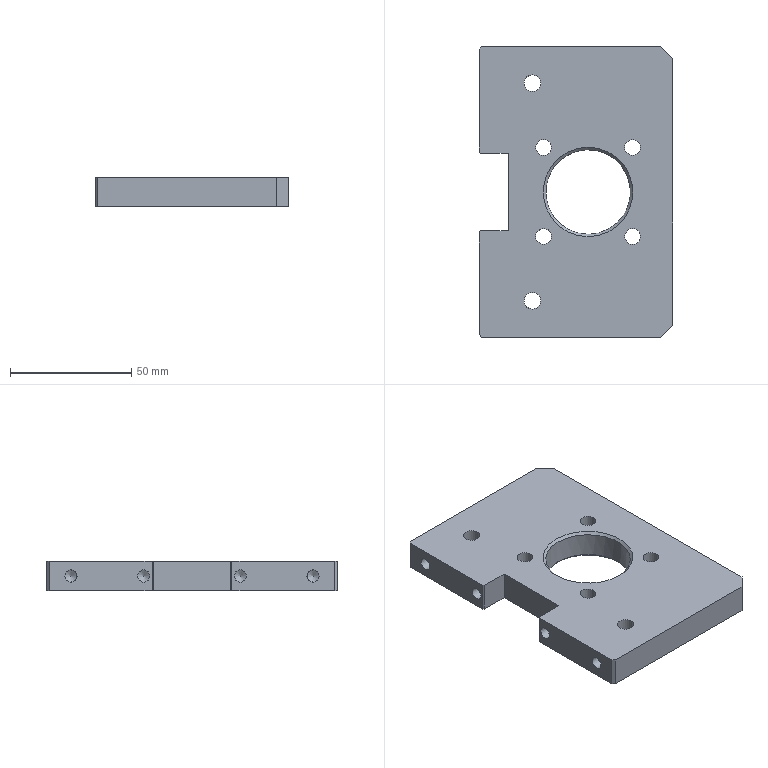NC program | NX | posted with a generic post | part box 80 x 120 x 12 mm
Whole program:
N10 G17 G21 G94 G90
(DRILLING , TOOL : D8A45)
N12 T06 M6
N14 G54
N16 G17 G0 G90 X-50. Y0. B0. C0. S3500 M3
N18 G43 Z30. H6
N20 G94 G81 G98 Z-2.6 F250. R3.
N22 X-20.
N24 X20.
N26 X50.
N28 G80
N30 G0 X50. Y0. Z30.
N32 M5
(DRILLING_1 , TOOL : 5.0ZT)
N34 T14 M6
N36 G54
N38 G17 G0 G90 X-50. Y0. B0. C0. S2000 M3
N40 G43 Z30. H14
N42 G94 G83 G98 Z-21.443 F200. Q3. R3.
N44 X-20.
N46 X20.
N48 X50.
N50 G80
N52 G0 X50. Y0. Z30.
N54 M5
(FLOOR_WALL_1 , TOOL : D10)
N56 T04 M6
N58 G54
N60 G17 G0 G90 X-1. Y12.5 B0. C0. S7000 M3
N62 G43 Z30. H4
N64 Z0.508
N66 G94 G1 Z-0.992 F1000.
N68 Y7.
N70 G3 X0. Y6. R1.
N72 G1 X10.9 F3000.
N74 Y-6.
N76 X-10.9
N78 Y6.
N80 X0.
N82 Y1.5
N84 X6.4
N86 Y-1.5
N88 X-6.4
N90 Y1.5
N92 X0.
N94 G3 X1. Y2.5 R1.
N96 G1 Z0.508
N98 G0 X-1. Y12.5 Z-0.483
N100 G1 Z-1.983 F1000.
N102 Y7.
N104 G3 X0. Y6. R1.
N106 G1 X10.9 F3000.
N108 Y-6.
N110 X-10.9
N112 Y6.
N114 X0.
N116 Y1.5
N118 X6.4
N120 Y-1.5
N122 X-6.4
N124 Y1.5
N126 X0.
N128 G3 X1. Y2.5 R1.
N130 G1 Z-0.483
N132 G0 X-1. Y12.5 Z-1.475
N134 G1 Z-2.975 F1000.
N136 Y7.
N138 G3 X0. Y6. R1.
N140 G1 X10.9 F3000.
N142 Y-6.
N144 X-10.9
N146 Y6.
N148 X0.
N150 Y1.5
N152 X6.4
N154 Y-1.5
N156 X-6.4
N158 Y1.5
N160 X0.
N162 G3 X1. Y2.5 R1.
N164 G1 Z-1.475
N166 G0 X-1. Y12.5 Z-2.467
N168 G1 Z-3.967 F1000.
N170 Y7.
N172 G3 X0. Y6. R1.
N174 G1 X10.9 F3000.
N176 Y-6.
N178 X-10.9
N180 Y6.
N182 X0.
N184 Y1.5
N186 X6.4
N188 Y-1.5
N190 X-6.4
N192 Y1.5
N194 X0.
N196 G3 X1. Y2.5 R1.
N198 G1 Z-2.467
N200 G0 X-1. Y12.5 Z-3.458
N202 G1 Z-4.958 F1000.
N204 Y7.
N206 G3 X0. Y6. R1.
N208 G1 X10.9 F3000.
N210 Y-6.
N212 X-10.9
N214 Y6.
N216 X0.
N218 Y1.5
N220 X6.4
N222 Y-1.5
N224 X-6.4
N226 Y1.5
N228 X0.
N230 G3 X1. Y2.5 R1.
N232 G1 Z-3.458
N234 G0 X-1. Y12.5 Z-4.45
N236 G1 Z-5.95 F1000.
N238 Y7.
N240 G3 X0. Y6. R1.
N242 G1 X10.9 F3000.
N244 Y-6.
N246 X-10.9
N248 Y6.
N250 X0.
N252 Y1.5
N254 X6.4
N256 Y-1.5
N258 X-6.4
N260 Y1.5
N262 X0.
N264 G3 X1. Y2.5 R1.
N266 G1 Z-4.45
N268 G0 X-1. Y12.5 Z-5.442
N270 G1 Z-6.942 F1000.
N272 Y7.
N274 G3 X0. Y6. R1.
N276 G1 X10.9 F3000.
N278 Y-6.
N280 X-10.9
N282 Y6.
N284 X0.
N286 Y1.5
N288 X6.4
N290 Y-1.5
N292 X-6.4
N294 Y1.5
N296 X0.
N298 G3 X1. Y2.5 R1.
N300 G1 Z-5.442
N302 G0 X-1. Y12.5 Z-6.433
N304 G1 Z-7.933 F1000.
N306 Y7.
N308 G3 X0. Y6. R1.
N310 G1 X10.9 F3000.
N312 Y-6.
N314 X-10.9
N316 Y6.
N318 X0.
N320 Y1.5
N322 X6.4
N324 Y-1.5
N326 X-6.4
N328 Y1.5
N330 X0.
N332 G3 X1. Y2.5 R1.
N334 G1 Z-6.433
N336 G0 X-1. Y12.5 Z-7.425
N338 G1 Z-8.925 F1000.
N340 Y7.
N342 G3 X0. Y6. R1.
N344 G1 X10.9 F3000.
N346 Y-6.
N348 X-10.9
N350 Y6.
N352 X0.
N354 Y1.5
N356 X6.4
N358 Y-1.5
N360 X-6.4
N362 Y1.5
N364 X0.
N366 G3 X1. Y2.5 R1.
N368 G1 Z-7.425
N370 G0 X-1. Y12.5 Z-8.417
N372 G1 Z-9.917 F1000.
N374 Y7.
N376 G3 X0. Y6. R1.
N378 G1 X10.9 F3000.
N380 Y-6.
N382 X-10.9
N384 Y6.
N386 X0.
N388 Y1.5
N390 X6.4
N392 Y-1.5
N394 X-6.4
N396 Y1.5
N398 X0.
N400 G3 X1. Y2.5 R1.
N402 G1 Z-8.417
N404 G0 X-1. Y12.5 Z-9.408
N406 G1 Z-10.908 F1000.
N408 Y7.
N410 G3 X0. Y6. R1.
N412 G1 X10.9 F3000.
N414 Y-6.
N416 X-10.9
N418 Y6.
N420 X0.
N422 Y1.5
N424 X6.4
N426 Y-1.5
N428 X-6.4
N430 Y1.5
N432 X0.
N434 G3 X1. Y2.5 R1.
N436 G1 Z-9.408
N438 G0 X-1. Y12.5 Z-10.4
N440 G1 Z-11.9 F1000.
N442 Y7.
N444 G3 X0. Y6. R1.
N446 G1 X10.9 F3000.
N448 Y-6.
N450 X-10.9
N452 Y6.
N454 X0.
N456 Y1.5
N458 X6.4
N460 Y-1.5
N462 X-6.4
N464 Y1.5
N466 X0.
N468 G3 X1. Y2.5 R1.
N470 G1 Z-10.4
N472 G0 Z30.
(FLOOR_WALL_1_COPY , TOOL : D10)
N474 X-9.497 Y-12.5
N476 Z-10.5
N478 G1 Z-12. F1000.
N480 Y-10.
N482 G3 X-10.497 Y-11. R1.
N484 G1 Y11. F1200.
N486 X-6.298
N488 Y-11.
N490 X-2.098
N492 Y11.
N494 X2.101
N496 Y-11.
N498 X6.301
N500 Y11.
N502 X10.5
N504 Y-11.
N506 G2 X9.5 Y-12. R1.
N508 G1 Y-12.5
N510 Z-10.5
N512 G0 Z-8.
N514 X10.
N516 Z-10.5
N518 G1 Z-12. F1000.
N520 Y-12.
N522 G3 X11. Y-11. R1.
N524 G1 Y11. F1200.
N526 G3 X10. Y12. R1.
N528 G1 Y12.5
N530 Z-10.5
N532 G0 Z-8.
N534 X-10.
N536 Z-10.5
N538 G1 Z-12. F1000.
N540 Y12.
N542 G3 X-11. Y11. R1.
N544 G1 Y-11. F1200.
N546 G3 X-10. Y-12. R1.
N548 G1 Y-12.5
N550 Z-10.5
N552 G0 Z30.
N554 M5
N556 M2